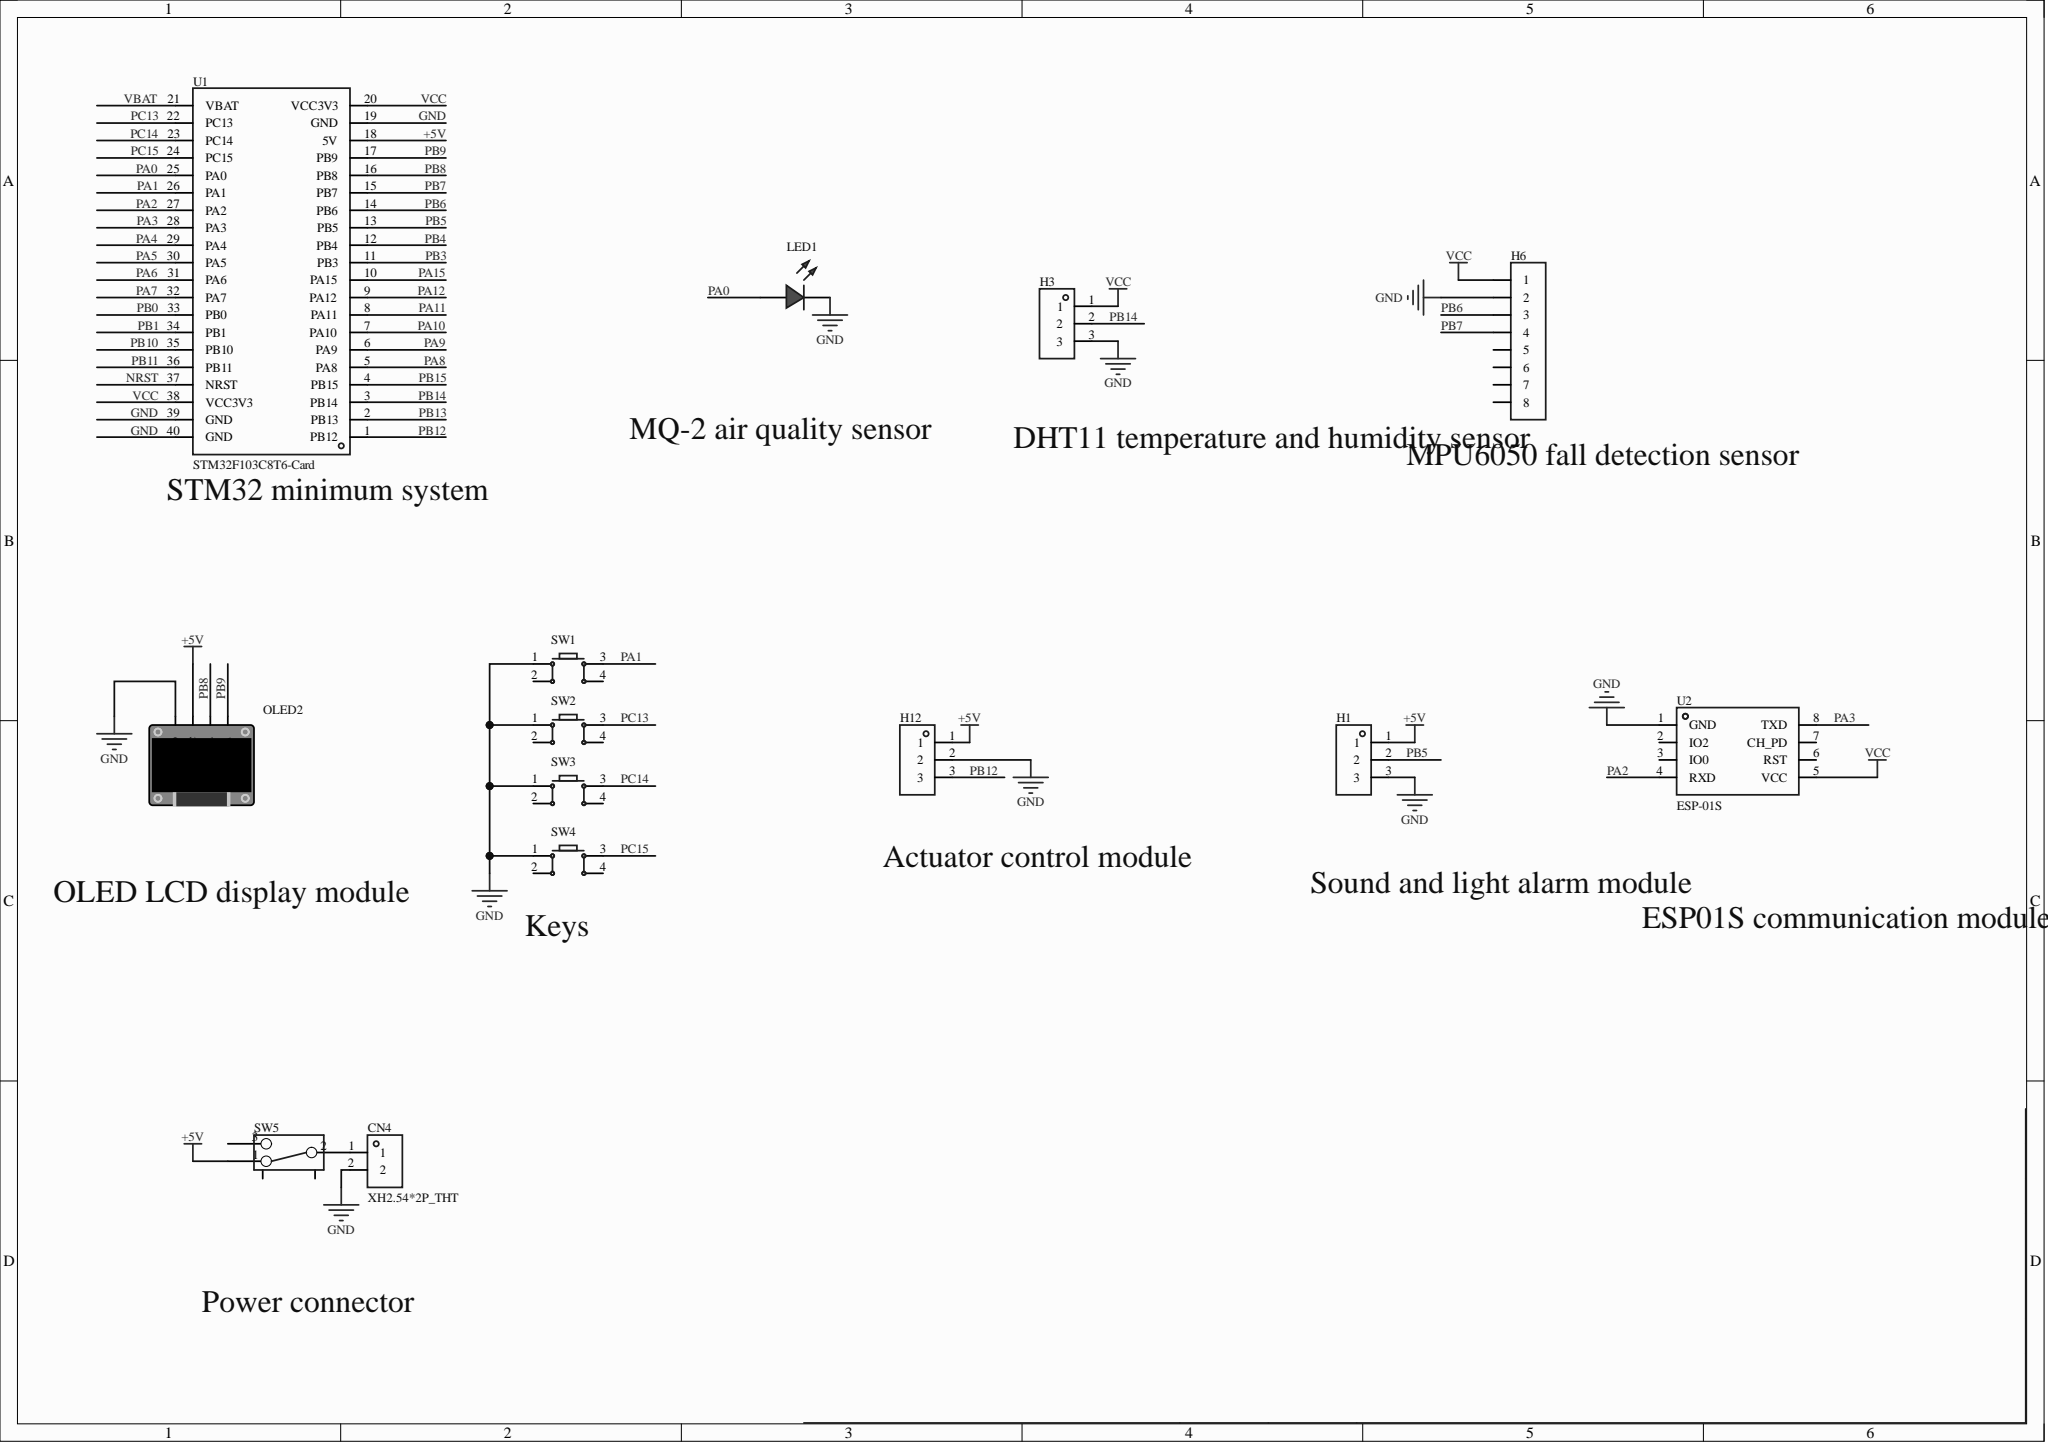Circuit board | Altium Designer | 14 parts | 18 nets
Bill of materials:
Comment,Description,Designator,Footprint,LibRef,Quantity
"XH2.54*2P_THT","","CN4","CONN-TH_2P-P2.50-XH2.54-2P","XH2.54*2P_直插","1"
"","","H1, H3, H12","HDR-TH_3P-P2.54-V-F","HDR-F_2.54_1x3P","3"
"","","H6","HDR-TH_8P-P2.54-V-F-1","HDR-F_2.54_1x8P","1"
"","","LED1","LED_TH-3mm","LED_TH-R_3mm","1"
"","","OLED2","0.96OLED_4P","0.96OLED模块_4P","1"
"","","SW1, SW2, SW3, SW4","SW-TH_4P-L6.0-W6.0-P4.50-LS6.5","Key_TH_6x6x6","4"
"","","SW5","拨动开关","拨动开关_正","1"
"STM32F103C8T6-Card","","U1","CONN-TH_L53.3-W22.9_STM32F103C8T6-CARD","STM32F103C8T6-Card","1"
"ESP-01S","","U2","WIFIM-TH_ESP-01S","ESP-01S_C111009","1"
Netlist (Protel format):
[
CN4
CONN-TH_2P-P2.50-XH2.54-2P
XH2.54*2P_THT



]
[
H1
HDR-TH_3P-P2.54-V-F




]
[
H3
HDR-TH_3P-P2.54-V-F




]
[
H6
HDR-TH_8P-P2.54-V-F-1




]
[
H12
HDR-TH_3P-P2.54-V-F




]
[
LED1
LED_TH-3mm




]
[
OLED2
0.96OLED_4P




]
[
SW1
SW-TH_4P-L6.0-W6.0-P4.50-LS6.5




]
[
SW2
SW-TH_4P-L6.0-W6.0-P4.50-LS6.5




]
[
SW3
SW-TH_4P-L6.0-W6.0-P4.50-LS6.5




]
[
SW4
SW-TH_4P-L6.0-W6.0-P4.50-LS6.5




]
[
SW5
拨动开关




]
[
U1
CONN-TH_L53.3-W22.9_STM32F103C8T6-CARD
STM32F103C8T6-Card



]
[
U2
WIFIM-TH_ESP-01S
ESP-01S



]
(
VCC
H3-1
H6-1
U1-20
U1-38
U2-5
)
(
PC15
SW4-3
U1-24
)
(
PC14
SW3-3
U1-23
)
(
PC13
SW2-3
U1-22
)
(
PB14
H3-2
U1-3
)
(
PB12
H12-3
U1-1
)
(
PB9
OLED2-4
U1-17
)
(
PB8
OLED2-3
U1-16
)
(
PB7
H6-4
U1-15
)
(
PB6
H6-3
U1-14
)
(
PB5
H1-2
U1-13
)
(
PA3
U1-28
U2-8
)
(
PA2
U1-27
U2-4
)
(
PA1
SW1-3
U1-26
)
(
PA0
LED1-1
U1-25
)
(
NetCN4_1
CN4-1
SW5-2
)
(
GND
CN4-2
H1-3
H3-3
H6-2
H12-2
LED1-2
OLED2-1
SW1-1
SW2-1
SW3-1
SW4-1
U1-19
U1-39
U1-40
U2-1
)
(
+5V
H1-1
H12-1
OLED2-2
SW5-1
U1-18
)